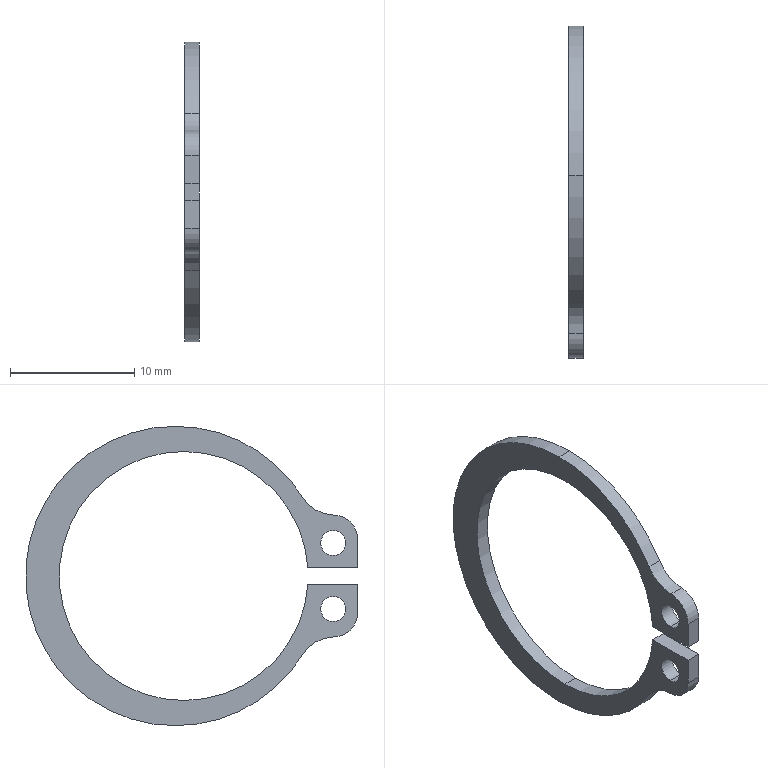Part | STEP file | 0230_012_STWN21 | 1 solid | 20 faces | box 1.2 x 26.7 x 24.05 mm | volume 188.679 mm3 | cylinder 14 | plane 6 | commonest cylinder face diameters 2 x4 20 x3 24.05 x3 4 x2 6 x2